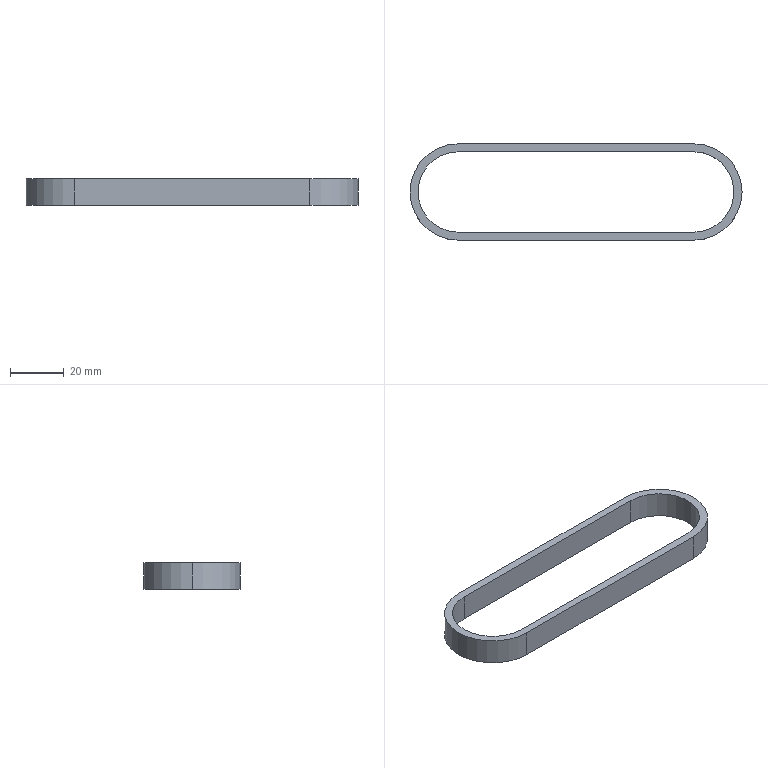Part | SolidWorks | features Extrusion 1, Shell 1 | 1 solid | 12 faces | box 124 x 36 x 10 mm | volume 8390 mm3 | cylinder 6 | plane 6 | commonest cylinder face diameters 30 x3 36 x3
STEP:
#1=CARTESIAN_POINT('',(-88.,15.,10.));
#2=VERTEX_POINT('',#1);
#3=CARTESIAN_POINT('',(-103.,0.,10.));
#4=VERTEX_POINT('',#3);
#5=CARTESIAN_POINT('',(-88.,0.,10.));
#6=DIRECTION('',(0.,0.,1.));
#7=DIRECTION('',(1.,0.,0.));
#8=AXIS2_PLACEMENT_3D('',#5,#6,#7);
#9=CIRCLE('',#8,15.);
#10=EDGE_CURVE('',#2,#4,#9,.T.);
#11=ORIENTED_EDGE('',*,*,#10,.T.);
#12=CARTESIAN_POINT('',(-103.,0.,0.));
#13=VERTEX_POINT('',#12);
#14=CARTESIAN_POINT('',(-103.,0.,10.));
#15=DIRECTION('',(0.,0.,-1.));
#16=VECTOR('',#15,1000.);
#17=LINE('',#14,#16);
#18=EDGE_CURVE('',#4,#13,#17,.T.);
#19=ORIENTED_EDGE('',*,*,#18,.T.);
#20=CARTESIAN_POINT('',(-88.,15.,0.));
#21=VERTEX_POINT('',#20);
#22=CARTESIAN_POINT('',(-88.,0.,0.));
#23=DIRECTION('',(0.,0.,1.));
#24=DIRECTION('',(1.,0.,0.));
#25=AXIS2_PLACEMENT_3D('',#22,#23,#24);
#26=CIRCLE('',#25,15.);
#27=EDGE_CURVE('',#21,#13,#26,.T.);
#28=ORIENTED_EDGE('',*,*,#27,.F.);
#29=CARTESIAN_POINT('',(-88.,15.,10.));
#30=DIRECTION('',(0.,0.,-1.));
#31=VECTOR('',#30,1000.);
#32=LINE('',#29,#31);
#33=EDGE_CURVE('',#2,#21,#32,.T.);
#34=ORIENTED_EDGE('',*,*,#33,.F.);
#35=EDGE_LOOP('',(#11,#19,#28,#34));
#36=FACE_OUTER_BOUND('',#35,.T.);
#37=CARTESIAN_POINT('',(-88.,0.,10.));
#38=DIRECTION('',(0.,0.,-1.));
#39=DIRECTION('',(-1.,0.,0.));
#40=AXIS2_PLACEMENT_3D('',#37,#38,#39);
#41=CYLINDRICAL_SURFACE('',#40,15.);
#42=ADVANCED_FACE('',(#36),#41,.F.);
#43=CARTESIAN_POINT('',(-106.,0.,10.));
#44=VERTEX_POINT('',#43);
#45=CARTESIAN_POINT('',(-88.,-18.,10.));
#46=VERTEX_POINT('',#45);
#47=CARTESIAN_POINT('',(-88.,0.,10.));
#48=DIRECTION('',(0.,0.,1.));
#49=DIRECTION('',(1.,0.,0.));
#50=AXIS2_PLACEMENT_3D('',#47,#48,#49);
#51=CIRCLE('',#50,18.);
#52=EDGE_CURVE('',#44,#46,#51,.T.);
#53=ORIENTED_EDGE('',*,*,#52,.F.);
#54=CARTESIAN_POINT('',(-106.,0.,0.));
#55=VERTEX_POINT('',#54);
#56=CARTESIAN_POINT('',(-106.,0.,10.));
#57=DIRECTION('',(0.,0.,-1.));
#58=VECTOR('',#57,1000.);
#59=LINE('',#56,#58);
#60=EDGE_CURVE('',#44,#55,#59,.T.);
#61=ORIENTED_EDGE('',*,*,#60,.T.);
#62=CARTESIAN_POINT('',(-88.,-18.,0.));
#63=VERTEX_POINT('',#62);
#64=CARTESIAN_POINT('',(-88.,0.,0.));
#65=DIRECTION('',(0.,0.,1.));
#66=DIRECTION('',(1.,0.,0.));
#67=AXIS2_PLACEMENT_3D('',#64,#65,#66);
#68=CIRCLE('',#67,18.);
#69=EDGE_CURVE('',#55,#63,#68,.T.);
#70=ORIENTED_EDGE('',*,*,#69,.T.);
#71=CARTESIAN_POINT('',(-88.,-18.,10.));
#72=DIRECTION('',(0.,0.,-1.));
#73=VECTOR('',#72,1000.);
#74=LINE('',#71,#73);
#75=EDGE_CURVE('',#46,#63,#74,.T.);
#76=ORIENTED_EDGE('',*,*,#75,.F.);
#77=EDGE_LOOP('',(#53,#61,#70,#76));
#78=FACE_OUTER_BOUND('',#77,.T.);
#79=CARTESIAN_POINT('',(-88.,0.,10.));
#80=DIRECTION('',(0.,0.,-1.));
#81=DIRECTION('',(-1.,0.,0.));
#82=AXIS2_PLACEMENT_3D('',#79,#80,#81);
#83=CYLINDRICAL_SURFACE('',#82,18.);
#84=ADVANCED_FACE('',(#78),#83,.T.);
#85=CARTESIAN_POINT('',(0.,-18.,0.));
#86=VERTEX_POINT('',#85);
#87=CARTESIAN_POINT('',(0.,18.,0.));
#88=VERTEX_POINT('',#87);
#89=CARTESIAN_POINT('',(0.,0.,0.));
#90=DIRECTION('',(0.,0.,1.));
#91=DIRECTION('',(1.,0.,0.));
#92=AXIS2_PLACEMENT_3D('',#89,#90,#91);
#93=CIRCLE('',#92,18.);
#94=EDGE_CURVE('',#86,#88,#93,.T.);
#95=ORIENTED_EDGE('',*,*,#94,.T.);
#96=CARTESIAN_POINT('',(0.,18.,10.));
#97=VERTEX_POINT('',#96);
#98=CARTESIAN_POINT('',(0.,18.,10.));
#99=DIRECTION('',(0.,0.,-1.));
#100=VECTOR('',#99,1000.);
#101=LINE('',#98,#100);
#102=EDGE_CURVE('',#97,#88,#101,.T.);
#103=ORIENTED_EDGE('',*,*,#102,.F.);
#104=CARTESIAN_POINT('',(0.,-18.,10.));
#105=VERTEX_POINT('',#104);
#106=CARTESIAN_POINT('',(0.,0.,10.));
#107=DIRECTION('',(0.,0.,1.));
#108=DIRECTION('',(1.,0.,0.));
#109=AXIS2_PLACEMENT_3D('',#106,#107,#108);
#110=CIRCLE('',#109,18.);
#111=EDGE_CURVE('',#105,#97,#110,.T.);
#112=ORIENTED_EDGE('',*,*,#111,.F.);
#113=CARTESIAN_POINT('',(0.,-18.,10.));
#114=DIRECTION('',(0.,0.,-1.));
#115=VECTOR('',#114,1000.);
#116=LINE('',#113,#115);
#117=EDGE_CURVE('',#105,#86,#116,.T.);
#118=ORIENTED_EDGE('',*,*,#117,.T.);
#119=EDGE_LOOP('',(#95,#103,#112,#118));
#120=FACE_OUTER_BOUND('',#119,.T.);
#121=CARTESIAN_POINT('',(0.,0.,10.));
#122=DIRECTION('',(0.,0.,-1.));
#123=DIRECTION('',(-1.,0.,0.));
#124=AXIS2_PLACEMENT_3D('',#121,#122,#123);
#125=CYLINDRICAL_SURFACE('',#124,18.);
#126=ADVANCED_FACE('',(#120),#125,.T.);
#127=CARTESIAN_POINT('',(-88.,18.,0.));
#128=VERTEX_POINT('',#127);
#129=CARTESIAN_POINT('',(0.,18.,0.));
#130=DIRECTION('',(-1.,0.,0.));
#131=VECTOR('',#130,1000.);
#132=LINE('',#129,#131);
#133=EDGE_CURVE('',#88,#128,#132,.T.);
#134=ORIENTED_EDGE('',*,*,#133,.T.);
#135=CARTESIAN_POINT('',(-88.,18.,10.));
#136=VERTEX_POINT('',#135);
#137=CARTESIAN_POINT('',(-88.,18.,10.));
#138=DIRECTION('',(0.,0.,-1.));
#139=VECTOR('',#138,1000.);
#140=LINE('',#137,#139);
#141=EDGE_CURVE('',#136,#128,#140,.T.);
#142=ORIENTED_EDGE('',*,*,#141,.F.);
#143=CARTESIAN_POINT('',(0.,18.,10.));
#144=DIRECTION('',(-1.,0.,0.));
#145=VECTOR('',#144,1000.);
#146=LINE('',#143,#145);
#147=EDGE_CURVE('',#97,#136,#146,.T.);
#148=ORIENTED_EDGE('',*,*,#147,.F.);
#149=ORIENTED_EDGE('',*,*,#102,.T.);
#150=EDGE_LOOP('',(#134,#142,#148,#149));
#151=FACE_OUTER_BOUND('',#150,.T.);
#152=CARTESIAN_POINT('',(0.,18.,10.));
#153=DIRECTION('',(0.,-1.,0.));
#154=DIRECTION('',(0.,0.,-1.));
#155=AXIS2_PLACEMENT_3D('',#152,#153,#154);
#156=PLANE('',#155);
#157=ADVANCED_FACE('',(#151),#156,.F.);
#158=ORIENTED_EDGE('',*,*,#60,.F.);
#159=CARTESIAN_POINT('',(-88.,0.,10.));
#160=DIRECTION('',(0.,0.,1.));
#161=DIRECTION('',(1.,0.,0.));
#162=AXIS2_PLACEMENT_3D('',#159,#160,#161);
#163=CIRCLE('',#162,18.);
#164=EDGE_CURVE('',#136,#44,#163,.T.);
#165=ORIENTED_EDGE('',*,*,#164,.F.);
#166=ORIENTED_EDGE('',*,*,#141,.T.);
#167=CARTESIAN_POINT('',(-88.,0.,0.));
#168=DIRECTION('',(0.,0.,1.));
#169=DIRECTION('',(1.,0.,0.));
#170=AXIS2_PLACEMENT_3D('',#167,#168,#169);
#171=CIRCLE('',#170,18.);
#172=EDGE_CURVE('',#128,#55,#171,.T.);
#173=ORIENTED_EDGE('',*,*,#172,.T.);
#174=EDGE_LOOP('',(#158,#165,#166,#173));
#175=FACE_OUTER_BOUND('',#174,.T.);
#176=CARTESIAN_POINT('',(-88.,0.,10.));
#177=DIRECTION('',(0.,0.,-1.));
#178=DIRECTION('',(-1.,0.,0.));
#179=AXIS2_PLACEMENT_3D('',#176,#177,#178);
#180=CYLINDRICAL_SURFACE('',#179,18.);
#181=ADVANCED_FACE('',(#175),#180,.T.);
#182=CARTESIAN_POINT('',(0.,-18.,0.));
#183=DIRECTION('',(1.,0.,0.));
#184=VECTOR('',#183,1000.);
#185=LINE('',#182,#184);
#186=EDGE_CURVE('',#63,#86,#185,.T.);
#187=ORIENTED_EDGE('',*,*,#186,.T.);
#188=ORIENTED_EDGE('',*,*,#117,.F.);
#189=CARTESIAN_POINT('',(0.,-18.,10.));
#190=DIRECTION('',(1.,0.,0.));
#191=VECTOR('',#190,1000.);
#192=LINE('',#189,#191);
#193=EDGE_CURVE('',#46,#105,#192,.T.);
#194=ORIENTED_EDGE('',*,*,#193,.F.);
#195=ORIENTED_EDGE('',*,*,#75,.T.);
#196=EDGE_LOOP('',(#187,#188,#194,#195));
#197=FACE_OUTER_BOUND('',#196,.T.);
#198=CARTESIAN_POINT('',(0.,-18.,10.));
#199=DIRECTION('',(0.,1.,0.));
#200=DIRECTION('',(0.,0.,1.));
#201=AXIS2_PLACEMENT_3D('',#198,#199,#200);
#202=PLANE('',#201);
#203=ADVANCED_FACE('',(#197),#202,.F.);
#204=CARTESIAN_POINT('',(0.,-15.,10.));
#205=VERTEX_POINT('',#204);
#206=CARTESIAN_POINT('',(0.,15.,10.));
#207=VERTEX_POINT('',#206);
#208=CARTESIAN_POINT('',(0.,0.,10.));
#209=DIRECTION('',(0.,0.,1.));
#210=DIRECTION('',(1.,0.,0.));
#211=AXIS2_PLACEMENT_3D('',#208,#209,#210);
#212=CIRCLE('',#211,15.);
#213=EDGE_CURVE('',#205,#207,#212,.T.);
#214=ORIENTED_EDGE('',*,*,#213,.F.);
#215=CARTESIAN_POINT('',(-88.,-15.,10.));
#216=VERTEX_POINT('',#215);
#217=CARTESIAN_POINT('',(0.,-15.,10.));
#218=DIRECTION('',(1.,0.,0.));
#219=VECTOR('',#218,1000.);
#220=LINE('',#217,#219);
#221=EDGE_CURVE('',#216,#205,#220,.T.);
#222=ORIENTED_EDGE('',*,*,#221,.F.);
#223=CARTESIAN_POINT('',(-88.,0.,10.));
#224=DIRECTION('',(0.,0.,1.));
#225=DIRECTION('',(1.,0.,0.));
#226=AXIS2_PLACEMENT_3D('',#223,#224,#225);
#227=CIRCLE('',#226,15.);
#228=EDGE_CURVE('',#4,#216,#227,.T.);
#229=ORIENTED_EDGE('',*,*,#228,.F.);
#230=ORIENTED_EDGE('',*,*,#10,.F.);
#231=CARTESIAN_POINT('',(0.,15.,10.));
#232=DIRECTION('',(-1.,0.,0.));
#233=VECTOR('',#232,1000.);
#234=LINE('',#231,#233);
#235=EDGE_CURVE('',#207,#2,#234,.T.);
#236=ORIENTED_EDGE('',*,*,#235,.F.);
#237=EDGE_LOOP('',(#214,#222,#229,#230,#236));
#238=FACE_BOUND('',#237,.T.);
#239=ORIENTED_EDGE('',*,*,#111,.T.);
#240=ORIENTED_EDGE('',*,*,#147,.T.);
#241=ORIENTED_EDGE('',*,*,#164,.T.);
#242=ORIENTED_EDGE('',*,*,#52,.T.);
#243=ORIENTED_EDGE('',*,*,#193,.T.);
#244=EDGE_LOOP('',(#239,#240,#241,#242,#243));
#245=FACE_OUTER_BOUND('',#244,.T.);
#246=CARTESIAN_POINT('',(0.,0.,10.));
#247=DIRECTION('',(0.,0.,1.));
#248=DIRECTION('',(1.,0.,0.));
#249=AXIS2_PLACEMENT_3D('',#246,#247,#248);
#250=PLANE('',#249);
#251=ADVANCED_FACE('',(#238,#245),#250,.T.);
#252=CARTESIAN_POINT('',(-88.,-15.,0.));
#253=VERTEX_POINT('',#252);
#254=CARTESIAN_POINT('',(0.,-15.,0.));
#255=VERTEX_POINT('',#254);
#256=CARTESIAN_POINT('',(0.,-15.,0.));
#257=DIRECTION('',(1.,0.,0.));
#258=VECTOR('',#257,1000.);
#259=LINE('',#256,#258);
#260=EDGE_CURVE('',#253,#255,#259,.T.);
#261=ORIENTED_EDGE('',*,*,#260,.T.);
#262=CARTESIAN_POINT('',(0.,15.,0.));
#263=VERTEX_POINT('',#262);
#264=CARTESIAN_POINT('',(0.,0.,0.));
#265=DIRECTION('',(0.,0.,1.));
#266=DIRECTION('',(1.,0.,0.));
#267=AXIS2_PLACEMENT_3D('',#264,#265,#266);
#268=CIRCLE('',#267,15.);
#269=EDGE_CURVE('',#255,#263,#268,.T.);
#270=ORIENTED_EDGE('',*,*,#269,.T.);
#271=CARTESIAN_POINT('',(0.,15.,0.));
#272=DIRECTION('',(-1.,0.,0.));
#273=VECTOR('',#272,1000.);
#274=LINE('',#271,#273);
#275=EDGE_CURVE('',#263,#21,#274,.T.);
#276=ORIENTED_EDGE('',*,*,#275,.T.);
#277=ORIENTED_EDGE('',*,*,#27,.T.);
#278=CARTESIAN_POINT('',(-88.,0.,0.));
#279=DIRECTION('',(0.,0.,1.));
#280=DIRECTION('',(1.,0.,0.));
#281=AXIS2_PLACEMENT_3D('',#278,#279,#280);
#282=CIRCLE('',#281,15.);
#283=EDGE_CURVE('',#13,#253,#282,.T.);
#284=ORIENTED_EDGE('',*,*,#283,.T.);
#285=EDGE_LOOP('',(#261,#270,#276,#277,#284));
#286=FACE_BOUND('',#285,.T.);
#287=ORIENTED_EDGE('',*,*,#94,.F.);
#288=ORIENTED_EDGE('',*,*,#186,.F.);
#289=ORIENTED_EDGE('',*,*,#69,.F.);
#290=ORIENTED_EDGE('',*,*,#172,.F.);
#291=ORIENTED_EDGE('',*,*,#133,.F.);
#292=EDGE_LOOP('',(#287,#288,#289,#290,#291));
#293=FACE_OUTER_BOUND('',#292,.T.);
#294=CARTESIAN_POINT('',(0.,0.,0.));
#295=DIRECTION('',(0.,0.,1.));
#296=DIRECTION('',(1.,0.,0.));
#297=AXIS2_PLACEMENT_3D('',#294,#295,#296);
#298=PLANE('',#297);
#299=ADVANCED_FACE('',(#286,#293),#298,.F.);
#300=ORIENTED_EDGE('',*,*,#269,.F.);
#301=CARTESIAN_POINT('',(0.,-15.,10.));
#302=DIRECTION('',(0.,0.,-1.));
#303=VECTOR('',#302,1000.);
#304=LINE('',#301,#303);
#305=EDGE_CURVE('',#205,#255,#304,.T.);
#306=ORIENTED_EDGE('',*,*,#305,.F.);
#307=ORIENTED_EDGE('',*,*,#213,.T.);
#308=CARTESIAN_POINT('',(0.,15.,10.));
#309=DIRECTION('',(0.,0.,-1.));
#310=VECTOR('',#309,1000.);
#311=LINE('',#308,#310);
#312=EDGE_CURVE('',#207,#263,#311,.T.);
#313=ORIENTED_EDGE('',*,*,#312,.T.);
#314=EDGE_LOOP('',(#300,#306,#307,#313));
#315=FACE_OUTER_BOUND('',#314,.T.);
#316=CARTESIAN_POINT('',(0.,0.,10.));
#317=DIRECTION('',(0.,0.,-1.));
#318=DIRECTION('',(-1.,0.,0.));
#319=AXIS2_PLACEMENT_3D('',#316,#317,#318);
#320=CYLINDRICAL_SURFACE('',#319,15.);
#321=ADVANCED_FACE('',(#315),#320,.F.);
#322=ORIENTED_EDGE('',*,*,#275,.F.);
#323=ORIENTED_EDGE('',*,*,#312,.F.);
#324=ORIENTED_EDGE('',*,*,#235,.T.);
#325=ORIENTED_EDGE('',*,*,#33,.T.);
#326=EDGE_LOOP('',(#322,#323,#324,#325));
#327=FACE_OUTER_BOUND('',#326,.T.);
#328=CARTESIAN_POINT('',(0.,15.,10.));
#329=DIRECTION('',(0.,-1.,0.));
#330=DIRECTION('',(0.,0.,-1.));
#331=AXIS2_PLACEMENT_3D('',#328,#329,#330);
#332=PLANE('',#331);
#333=ADVANCED_FACE('',(#327),#332,.T.);
#334=ORIENTED_EDGE('',*,*,#18,.F.);
#335=ORIENTED_EDGE('',*,*,#228,.T.);
#336=CARTESIAN_POINT('',(-88.,-15.,10.));
#337=DIRECTION('',(0.,0.,-1.));
#338=VECTOR('',#337,1000.);
#339=LINE('',#336,#338);
#340=EDGE_CURVE('',#216,#253,#339,.T.);
#341=ORIENTED_EDGE('',*,*,#340,.T.);
#342=ORIENTED_EDGE('',*,*,#283,.F.);
#343=EDGE_LOOP('',(#334,#335,#341,#342));
#344=FACE_OUTER_BOUND('',#343,.T.);
#345=CARTESIAN_POINT('',(-88.,0.,10.));
#346=DIRECTION('',(0.,0.,-1.));
#347=DIRECTION('',(-1.,0.,0.));
#348=AXIS2_PLACEMENT_3D('',#345,#346,#347);
#349=CYLINDRICAL_SURFACE('',#348,15.);
#350=ADVANCED_FACE('',(#344),#349,.F.);
#351=ORIENTED_EDGE('',*,*,#260,.F.);
#352=ORIENTED_EDGE('',*,*,#340,.F.);
#353=ORIENTED_EDGE('',*,*,#221,.T.);
#354=ORIENTED_EDGE('',*,*,#305,.T.);
#355=EDGE_LOOP('',(#351,#352,#353,#354));
#356=FACE_OUTER_BOUND('',#355,.T.);
#357=CARTESIAN_POINT('',(0.,-15.,10.));
#358=DIRECTION('',(0.,1.,0.));
#359=DIRECTION('',(0.,0.,1.));
#360=AXIS2_PLACEMENT_3D('',#357,#358,#359);
#361=PLANE('',#360);
#362=ADVANCED_FACE('',(#356),#361,.T.);
#363=CLOSED_SHELL('',(#42,#84,#126,#157,#181,#203,#251,#299,#321,#333,#350,#362));
#364=MANIFOLD_SOLID_BREP('',#363);
#365=CARTESIAN_POINT('',(0.,0.,0.));
#366=DIRECTION('',(0.,0.,1.));
#367=DIRECTION('',(1.,0.,0.));
#368=AXIS2_PLACEMENT_3D('',#365,#366,#367);
#369=(LENGTH_UNIT()NAMED_UNIT(*)SI_UNIT(.MILLI.,.METRE.));
#370=UNCERTAINTY_MEASURE_WITH_UNIT(LENGTH_MEASURE(0.00001),#369,'','');
#371=(NAMED_UNIT(*)PLANE_ANGLE_UNIT()SI_UNIT($,.RADIAN.));
#372=(NAMED_UNIT(*)SI_UNIT($,.STERADIAN.)SOLID_ANGLE_UNIT());
#373=(GEOMETRIC_REPRESENTATION_CONTEXT(3)GLOBAL_UNCERTAINTY_ASSIGNED_CONTEXT((#370))GLOBAL_UNIT_ASSIGNED_CONTEXT((#369,#371,#372))REPRESENTATION_CONTEXT('',''));
#374=ADVANCED_BREP_SHAPE_REPRESENTATION('',(#364,#368),#373);